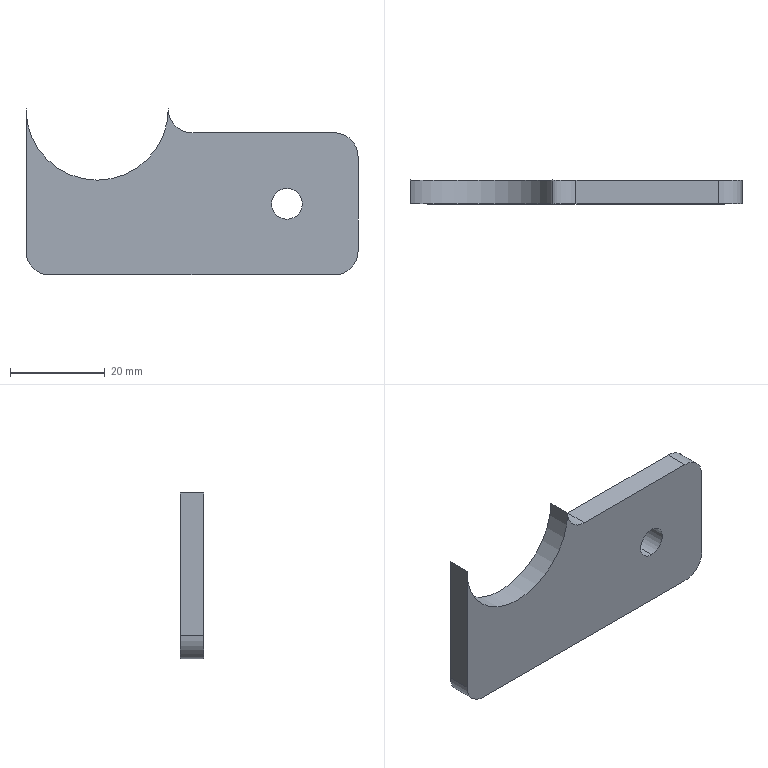Part | SolidWorks | features Cut 1, Extrusion 1, Fillet 1, ICE 1 | 1 solid | 13 faces | box 70 x 5 x 35 mm | volume 9263 mm3 | cylinder 7 | plane 6 | commonest cylinder face diameters 10 x4 6.5 x2 30 x1
STEP:
#1=CARTESIAN_POINT('',(40.,205.,-23.25));
#2=VERTEX_POINT('',#1);
#3=CARTESIAN_POINT('',(40.,205.,-16.75));
#4=VERTEX_POINT('',#3);
#5=CARTESIAN_POINT('',(40.,205.,-20.));
#6=DIRECTION('',(0.,1.,0.));
#7=DIRECTION('',(0.,0.,1.));
#8=AXIS2_PLACEMENT_3D('',#5,#6,#7);
#9=CIRCLE('',#8,3.25);
#10=EDGE_CURVE('',#2,#4,#9,.T.);
#11=ORIENTED_EDGE('',*,*,#10,.F.);
#12=CARTESIAN_POINT('',(40.,210.,-23.25));
#13=VERTEX_POINT('',#12);
#14=CARTESIAN_POINT('',(40.,205.,-23.25));
#15=DIRECTION('',(0.,1.,0.));
#16=VECTOR('',#15,1000.);
#17=LINE('',#14,#16);
#18=EDGE_CURVE('',#2,#13,#17,.T.);
#19=ORIENTED_EDGE('',*,*,#18,.T.);
#20=CARTESIAN_POINT('',(40.,210.,-16.75));
#21=VERTEX_POINT('',#20);
#22=CARTESIAN_POINT('',(40.,210.,-20.));
#23=DIRECTION('',(0.,1.,0.));
#24=DIRECTION('',(0.,0.,1.));
#25=AXIS2_PLACEMENT_3D('',#22,#23,#24);
#26=CIRCLE('',#25,3.25);
#27=EDGE_CURVE('',#13,#21,#26,.T.);
#28=ORIENTED_EDGE('',*,*,#27,.T.);
#29=CARTESIAN_POINT('',(40.,205.,-16.75));
#30=DIRECTION('',(0.,1.,0.));
#31=VECTOR('',#30,1000.);
#32=LINE('',#29,#31);
#33=EDGE_CURVE('',#4,#21,#32,.T.);
#34=ORIENTED_EDGE('',*,*,#33,.F.);
#35=EDGE_LOOP('',(#11,#19,#28,#34));
#36=FACE_OUTER_BOUND('',#35,.T.);
#37=CARTESIAN_POINT('',(40.,205.,-20.));
#38=DIRECTION('',(0.,1.,0.));
#39=DIRECTION('',(0.,0.,1.));
#40=AXIS2_PLACEMENT_3D('',#37,#38,#39);
#41=CYLINDRICAL_SURFACE('',#40,3.25);
#42=ADVANCED_FACE('',(#36),#41,.F.);
#43=CARTESIAN_POINT('',(20.,210.,-5.));
#44=VERTEX_POINT('',#43);
#45=CARTESIAN_POINT('',(50.,210.,-5.));
#46=VERTEX_POINT('',#45);
#47=CARTESIAN_POINT('',(14.142,210.,-5.));
#48=DIRECTION('',(1.,0.,0.));
#49=VECTOR('',#48,1000.);
#50=LINE('',#47,#49);
#51=EDGE_CURVE('',#44,#46,#50,.T.);
#52=ORIENTED_EDGE('',*,*,#51,.F.);
#53=CARTESIAN_POINT('',(20.,205.,-5.));
#54=VERTEX_POINT('',#53);
#55=CARTESIAN_POINT('',(20.,205.,-5.));
#56=DIRECTION('',(0.,1.,0.));
#57=VECTOR('',#56,1000.);
#58=LINE('',#55,#57);
#59=EDGE_CURVE('',#54,#44,#58,.T.);
#60=ORIENTED_EDGE('',*,*,#59,.F.);
#61=CARTESIAN_POINT('',(50.,205.,-5.));
#62=VERTEX_POINT('',#61);
#63=CARTESIAN_POINT('',(14.142,205.,-5.));
#64=DIRECTION('',(1.,0.,0.));
#65=VECTOR('',#64,1000.);
#66=LINE('',#63,#65);
#67=EDGE_CURVE('',#54,#62,#66,.T.);
#68=ORIENTED_EDGE('',*,*,#67,.T.);
#69=CARTESIAN_POINT('',(50.,205.,-5.));
#70=DIRECTION('',(0.,1.,0.));
#71=VECTOR('',#70,1000.);
#72=LINE('',#69,#71);
#73=EDGE_CURVE('',#62,#46,#72,.T.);
#74=ORIENTED_EDGE('',*,*,#73,.T.);
#75=EDGE_LOOP('',(#52,#60,#68,#74));
#76=FACE_OUTER_BOUND('',#75,.T.);
#77=CARTESIAN_POINT('',(14.142,205.,-5.));
#78=DIRECTION('',(0.,0.,1.));
#79=DIRECTION('',(1.,0.,0.));
#80=AXIS2_PLACEMENT_3D('',#77,#78,#79);
#81=PLANE('',#80);
#82=ADVANCED_FACE('',(#76),#81,.T.);
#83=CARTESIAN_POINT('',(-15.,210.,0.));
#84=VERTEX_POINT('',#83);
#85=CARTESIAN_POINT('',(15.,210.,0.));
#86=VERTEX_POINT('',#85);
#87=CARTESIAN_POINT('',(0.,210.,0.));
#88=DIRECTION('',(0.,-1.,0.));
#89=DIRECTION('',(0.,0.,1.));
#90=AXIS2_PLACEMENT_3D('',#87,#88,#89);
#91=CIRCLE('',#90,15.);
#92=EDGE_CURVE('',#84,#86,#91,.T.);
#93=ORIENTED_EDGE('',*,*,#92,.F.);
#94=CARTESIAN_POINT('',(-15.,205.,0.));
#95=VERTEX_POINT('',#94);
#96=CARTESIAN_POINT('',(-15.,205.,0.));
#97=DIRECTION('',(0.,1.,0.));
#98=VECTOR('',#97,1000.);
#99=LINE('',#96,#98);
#100=EDGE_CURVE('',#95,#84,#99,.T.);
#101=ORIENTED_EDGE('',*,*,#100,.F.);
#102=CARTESIAN_POINT('',(15.,205.,0.));
#103=VERTEX_POINT('',#102);
#104=CARTESIAN_POINT('',(0.,205.,0.));
#105=DIRECTION('',(0.,-1.,0.));
#106=DIRECTION('',(0.,0.,1.));
#107=AXIS2_PLACEMENT_3D('',#104,#105,#106);
#108=CIRCLE('',#107,15.);
#109=EDGE_CURVE('',#95,#103,#108,.T.);
#110=ORIENTED_EDGE('',*,*,#109,.T.);
#111=CARTESIAN_POINT('',(15.,205.,0.));
#112=DIRECTION('',(0.,1.,0.));
#113=VECTOR('',#112,1000.);
#114=LINE('',#111,#113);
#115=EDGE_CURVE('',#103,#86,#114,.T.);
#116=ORIENTED_EDGE('',*,*,#115,.T.);
#117=EDGE_LOOP('',(#93,#101,#110,#116));
#118=FACE_OUTER_BOUND('',#117,.T.);
#119=CARTESIAN_POINT('',(0.,205.,0.));
#120=DIRECTION('',(0.,1.,0.));
#121=DIRECTION('',(0.,0.,1.));
#122=AXIS2_PLACEMENT_3D('',#119,#120,#121);
#123=CYLINDRICAL_SURFACE('',#122,15.);
#124=ADVANCED_FACE('',(#118),#123,.F.);
#125=CARTESIAN_POINT('',(-15.,210.,-30.));
#126=VERTEX_POINT('',#125);
#127=CARTESIAN_POINT('',(-15.,210.,0.));
#128=DIRECTION('',(0.,0.,1.));
#129=VECTOR('',#128,1000.);
#130=LINE('',#127,#129);
#131=EDGE_CURVE('',#126,#84,#130,.T.);
#132=ORIENTED_EDGE('',*,*,#131,.F.);
#133=CARTESIAN_POINT('',(-15.,205.,-30.));
#134=VERTEX_POINT('',#133);
#135=CARTESIAN_POINT('',(-15.,205.,-30.));
#136=DIRECTION('',(0.,-1.,0.));
#137=VECTOR('',#136,1000.);
#138=LINE('',#135,#137);
#139=EDGE_CURVE('',#126,#134,#138,.T.);
#140=ORIENTED_EDGE('',*,*,#139,.T.);
#141=CARTESIAN_POINT('',(-15.,205.,0.));
#142=DIRECTION('',(0.,0.,1.));
#143=VECTOR('',#142,1000.);
#144=LINE('',#141,#143);
#145=EDGE_CURVE('',#134,#95,#144,.T.);
#146=ORIENTED_EDGE('',*,*,#145,.T.);
#147=ORIENTED_EDGE('',*,*,#100,.T.);
#148=EDGE_LOOP('',(#132,#140,#146,#147));
#149=FACE_OUTER_BOUND('',#148,.T.);
#150=CARTESIAN_POINT('',(-15.,205.,0.));
#151=DIRECTION('',(-1.,0.,0.));
#152=DIRECTION('',(0.,0.,1.));
#153=AXIS2_PLACEMENT_3D('',#150,#151,#152);
#154=PLANE('',#153);
#155=ADVANCED_FACE('',(#149),#154,.T.);
#156=CARTESIAN_POINT('',(50.,205.,-35.));
#157=VERTEX_POINT('',#156);
#158=CARTESIAN_POINT('',(-10.,205.,-35.));
#159=VERTEX_POINT('',#158);
#160=CARTESIAN_POINT('',(-15.,205.,-35.));
#161=DIRECTION('',(-1.,0.,0.));
#162=VECTOR('',#161,1000.);
#163=LINE('',#160,#162);
#164=EDGE_CURVE('',#157,#159,#163,.T.);
#165=ORIENTED_EDGE('',*,*,#164,.T.);
#166=CARTESIAN_POINT('',(-10.,210.,-35.));
#167=VERTEX_POINT('',#166);
#168=CARTESIAN_POINT('',(-10.,205.,-35.));
#169=DIRECTION('',(0.,1.,0.));
#170=VECTOR('',#169,1000.);
#171=LINE('',#168,#170);
#172=EDGE_CURVE('',#159,#167,#171,.T.);
#173=ORIENTED_EDGE('',*,*,#172,.T.);
#174=CARTESIAN_POINT('',(50.,210.,-35.));
#175=VERTEX_POINT('',#174);
#176=CARTESIAN_POINT('',(-15.,210.,-35.));
#177=DIRECTION('',(-1.,0.,0.));
#178=VECTOR('',#177,1000.);
#179=LINE('',#176,#178);
#180=EDGE_CURVE('',#175,#167,#179,.T.);
#181=ORIENTED_EDGE('',*,*,#180,.F.);
#182=CARTESIAN_POINT('',(50.,205.,-35.));
#183=DIRECTION('',(0.,-1.,0.));
#184=VECTOR('',#183,1000.);
#185=LINE('',#182,#184);
#186=EDGE_CURVE('',#175,#157,#185,.T.);
#187=ORIENTED_EDGE('',*,*,#186,.T.);
#188=EDGE_LOOP('',(#165,#173,#181,#187));
#189=FACE_OUTER_BOUND('',#188,.T.);
#190=CARTESIAN_POINT('',(-15.,205.,-35.));
#191=DIRECTION('',(0.,0.,-1.));
#192=DIRECTION('',(-1.,0.,0.));
#193=AXIS2_PLACEMENT_3D('',#190,#191,#192);
#194=PLANE('',#193);
#195=ADVANCED_FACE('',(#189),#194,.T.);
#196=CARTESIAN_POINT('',(55.,210.,-10.));
#197=VERTEX_POINT('',#196);
#198=CARTESIAN_POINT('',(55.,210.,-30.));
#199=VERTEX_POINT('',#198);
#200=CARTESIAN_POINT('',(55.,210.,-5.));
#201=DIRECTION('',(0.,0.,-1.));
#202=VECTOR('',#201,1000.);
#203=LINE('',#200,#202);
#204=EDGE_CURVE('',#197,#199,#203,.T.);
#205=ORIENTED_EDGE('',*,*,#204,.F.);
#206=CARTESIAN_POINT('',(55.,205.,-10.));
#207=VERTEX_POINT('',#206);
#208=CARTESIAN_POINT('',(55.,205.,-10.));
#209=DIRECTION('',(0.,-1.,0.));
#210=VECTOR('',#209,1000.);
#211=LINE('',#208,#210);
#212=EDGE_CURVE('',#197,#207,#211,.T.);
#213=ORIENTED_EDGE('',*,*,#212,.T.);
#214=CARTESIAN_POINT('',(55.,205.,-30.));
#215=VERTEX_POINT('',#214);
#216=CARTESIAN_POINT('',(55.,205.,-5.));
#217=DIRECTION('',(0.,0.,-1.));
#218=VECTOR('',#217,1000.);
#219=LINE('',#216,#218);
#220=EDGE_CURVE('',#207,#215,#219,.T.);
#221=ORIENTED_EDGE('',*,*,#220,.T.);
#222=CARTESIAN_POINT('',(55.,205.,-30.));
#223=DIRECTION('',(0.,1.,0.));
#224=VECTOR('',#223,1000.);
#225=LINE('',#222,#224);
#226=EDGE_CURVE('',#215,#199,#225,.T.);
#227=ORIENTED_EDGE('',*,*,#226,.T.);
#228=EDGE_LOOP('',(#205,#213,#221,#227));
#229=FACE_OUTER_BOUND('',#228,.T.);
#230=CARTESIAN_POINT('',(55.,205.,-5.));
#231=DIRECTION('',(1.,0.,0.));
#232=DIRECTION('',(0.,0.,-1.));
#233=AXIS2_PLACEMENT_3D('',#230,#231,#232);
#234=PLANE('',#233);
#235=ADVANCED_FACE('',(#229),#234,.T.);
#236=CARTESIAN_POINT('',(40.,205.,-20.));
#237=DIRECTION('',(0.,1.,0.));
#238=DIRECTION('',(0.,0.,1.));
#239=AXIS2_PLACEMENT_3D('',#236,#237,#238);
#240=CIRCLE('',#239,3.25);
#241=EDGE_CURVE('',#4,#2,#240,.T.);
#242=ORIENTED_EDGE('',*,*,#241,.T.);
#243=ORIENTED_EDGE('',*,*,#10,.T.);
#244=EDGE_LOOP('',(#242,#243));
#245=FACE_BOUND('',#244,.T.);
#246=ORIENTED_EDGE('',*,*,#220,.F.);
#247=CARTESIAN_POINT('',(50.,205.,-10.));
#248=DIRECTION('',(0.,-1.,0.));
#249=DIRECTION('',(0.,0.,1.));
#250=AXIS2_PLACEMENT_3D('',#247,#248,#249);
#251=CIRCLE('',#250,5.);
#252=EDGE_CURVE('',#207,#62,#251,.T.);
#253=ORIENTED_EDGE('',*,*,#252,.T.);
#254=ORIENTED_EDGE('',*,*,#67,.F.);
#255=CARTESIAN_POINT('',(20.,205.,0.));
#256=DIRECTION('',(0.,-1.,0.));
#257=DIRECTION('',(0.,0.,1.));
#258=AXIS2_PLACEMENT_3D('',#255,#256,#257);
#259=CIRCLE('',#258,5.);
#260=EDGE_CURVE('',#103,#54,#259,.T.);
#261=ORIENTED_EDGE('',*,*,#260,.F.);
#262=ORIENTED_EDGE('',*,*,#109,.F.);
#263=ORIENTED_EDGE('',*,*,#145,.F.);
#264=CARTESIAN_POINT('',(-10.,205.,-30.));
#265=DIRECTION('',(0.,-1.,0.));
#266=DIRECTION('',(0.,0.,1.));
#267=AXIS2_PLACEMENT_3D('',#264,#265,#266);
#268=CIRCLE('',#267,5.);
#269=EDGE_CURVE('',#134,#159,#268,.T.);
#270=ORIENTED_EDGE('',*,*,#269,.T.);
#271=ORIENTED_EDGE('',*,*,#164,.F.);
#272=CARTESIAN_POINT('',(50.,205.,-30.));
#273=DIRECTION('',(0.,-1.,0.));
#274=DIRECTION('',(0.,0.,1.));
#275=AXIS2_PLACEMENT_3D('',#272,#273,#274);
#276=CIRCLE('',#275,5.);
#277=EDGE_CURVE('',#157,#215,#276,.T.);
#278=ORIENTED_EDGE('',*,*,#277,.T.);
#279=EDGE_LOOP('',(#246,#253,#254,#261,#262,#263,#270,#271,#278));
#280=FACE_OUTER_BOUND('',#279,.T.);
#281=CARTESIAN_POINT('',(0.,205.,0.));
#282=DIRECTION('',(0.,1.,0.));
#283=DIRECTION('',(0.,0.,1.));
#284=AXIS2_PLACEMENT_3D('',#281,#282,#283);
#285=PLANE('',#284);
#286=ADVANCED_FACE('',(#245,#280),#285,.F.);
#287=CARTESIAN_POINT('',(40.,210.,-20.));
#288=DIRECTION('',(0.,1.,0.));
#289=DIRECTION('',(0.,0.,1.));
#290=AXIS2_PLACEMENT_3D('',#287,#288,#289);
#291=CIRCLE('',#290,3.25);
#292=EDGE_CURVE('',#21,#13,#291,.T.);
#293=ORIENTED_EDGE('',*,*,#292,.F.);
#294=ORIENTED_EDGE('',*,*,#27,.F.);
#295=EDGE_LOOP('',(#293,#294));
#296=FACE_BOUND('',#295,.T.);
#297=ORIENTED_EDGE('',*,*,#92,.T.);
#298=CARTESIAN_POINT('',(20.,210.,0.));
#299=DIRECTION('',(0.,-1.,0.));
#300=DIRECTION('',(0.,0.,1.));
#301=AXIS2_PLACEMENT_3D('',#298,#299,#300);
#302=CIRCLE('',#301,5.);
#303=EDGE_CURVE('',#86,#44,#302,.T.);
#304=ORIENTED_EDGE('',*,*,#303,.T.);
#305=ORIENTED_EDGE('',*,*,#51,.T.);
#306=CARTESIAN_POINT('',(50.,210.,-10.));
#307=DIRECTION('',(0.,1.,0.));
#308=DIRECTION('',(0.,0.,1.));
#309=AXIS2_PLACEMENT_3D('',#306,#307,#308);
#310=CIRCLE('',#309,5.);
#311=EDGE_CURVE('',#46,#197,#310,.T.);
#312=ORIENTED_EDGE('',*,*,#311,.T.);
#313=ORIENTED_EDGE('',*,*,#204,.T.);
#314=CARTESIAN_POINT('',(50.,210.,-30.));
#315=DIRECTION('',(0.,1.,0.));
#316=DIRECTION('',(0.,0.,1.));
#317=AXIS2_PLACEMENT_3D('',#314,#315,#316);
#318=CIRCLE('',#317,5.);
#319=EDGE_CURVE('',#199,#175,#318,.T.);
#320=ORIENTED_EDGE('',*,*,#319,.T.);
#321=ORIENTED_EDGE('',*,*,#180,.T.);
#322=CARTESIAN_POINT('',(-10.,210.,-30.));
#323=DIRECTION('',(0.,1.,0.));
#324=DIRECTION('',(0.,0.,1.));
#325=AXIS2_PLACEMENT_3D('',#322,#323,#324);
#326=CIRCLE('',#325,5.);
#327=EDGE_CURVE('',#167,#126,#326,.T.);
#328=ORIENTED_EDGE('',*,*,#327,.T.);
#329=ORIENTED_EDGE('',*,*,#131,.T.);
#330=EDGE_LOOP('',(#297,#304,#305,#312,#313,#320,#321,#328,#329));
#331=FACE_OUTER_BOUND('',#330,.T.);
#332=CARTESIAN_POINT('',(0.,210.,0.));
#333=DIRECTION('',(0.,1.,0.));
#334=DIRECTION('',(0.,0.,1.));
#335=AXIS2_PLACEMENT_3D('',#332,#333,#334);
#336=PLANE('',#335);
#337=ADVANCED_FACE('',(#296,#331),#336,.T.);
#338=ORIENTED_EDGE('',*,*,#252,.F.);
#339=ORIENTED_EDGE('',*,*,#212,.F.);
#340=ORIENTED_EDGE('',*,*,#311,.F.);
#341=ORIENTED_EDGE('',*,*,#73,.F.);
#342=EDGE_LOOP('',(#338,#339,#340,#341));
#343=FACE_OUTER_BOUND('',#342,.T.);
#344=CARTESIAN_POINT('',(50.,205.,-10.));
#345=DIRECTION('',(0.,1.,0.));
#346=DIRECTION('',(0.,0.,1.));
#347=AXIS2_PLACEMENT_3D('',#344,#345,#346);
#348=CYLINDRICAL_SURFACE('',#347,5.);
#349=ADVANCED_FACE('',(#343),#348,.T.);
#350=ORIENTED_EDGE('',*,*,#269,.F.);
#351=ORIENTED_EDGE('',*,*,#139,.F.);
#352=ORIENTED_EDGE('',*,*,#327,.F.);
#353=ORIENTED_EDGE('',*,*,#172,.F.);
#354=EDGE_LOOP('',(#350,#351,#352,#353));
#355=FACE_OUTER_BOUND('',#354,.T.);
#356=CARTESIAN_POINT('',(-10.,205.,-30.));
#357=DIRECTION('',(0.,1.,0.));
#358=DIRECTION('',(0.,0.,1.));
#359=AXIS2_PLACEMENT_3D('',#356,#357,#358);
#360=CYLINDRICAL_SURFACE('',#359,5.);
#361=ADVANCED_FACE('',(#355),#360,.T.);
#362=ORIENTED_EDGE('',*,*,#277,.F.);
#363=ORIENTED_EDGE('',*,*,#186,.F.);
#364=ORIENTED_EDGE('',*,*,#319,.F.);
#365=ORIENTED_EDGE('',*,*,#226,.F.);
#366=EDGE_LOOP('',(#362,#363,#364,#365));
#367=FACE_OUTER_BOUND('',#366,.T.);
#368=CARTESIAN_POINT('',(50.,205.,-30.));
#369=DIRECTION('',(0.,1.,0.));
#370=DIRECTION('',(0.,0.,1.));
#371=AXIS2_PLACEMENT_3D('',#368,#369,#370);
#372=CYLINDRICAL_SURFACE('',#371,5.);
#373=ADVANCED_FACE('',(#367),#372,.T.);
#374=ORIENTED_EDGE('',*,*,#18,.F.);
#375=ORIENTED_EDGE('',*,*,#241,.F.);
#376=ORIENTED_EDGE('',*,*,#33,.T.);
#377=ORIENTED_EDGE('',*,*,#292,.T.);
#378=EDGE_LOOP('',(#374,#375,#376,#377));
#379=FACE_OUTER_BOUND('',#378,.T.);
#380=CARTESIAN_POINT('',(40.,205.,-20.));
#381=DIRECTION('',(0.,1.,0.));
#382=DIRECTION('',(0.,0.,1.));
#383=AXIS2_PLACEMENT_3D('',#380,#381,#382);
#384=CYLINDRICAL_SURFACE('',#383,3.25);
#385=ADVANCED_FACE('',(#379),#384,.F.);
#386=ORIENTED_EDGE('',*,*,#303,.F.);
#387=ORIENTED_EDGE('',*,*,#115,.F.);
#388=ORIENTED_EDGE('',*,*,#260,.T.);
#389=ORIENTED_EDGE('',*,*,#59,.T.);
#390=EDGE_LOOP('',(#386,#387,#388,#389));
#391=FACE_OUTER_BOUND('',#390,.T.);
#392=CARTESIAN_POINT('',(20.,205.,0.));
#393=DIRECTION('',(0.,1.,0.));
#394=DIRECTION('',(0.,0.,1.));
#395=AXIS2_PLACEMENT_3D('',#392,#393,#394);
#396=CYLINDRICAL_SURFACE('',#395,5.);
#397=ADVANCED_FACE('',(#391),#396,.F.);
#398=CLOSED_SHELL('',(#42,#82,#124,#155,#195,#235,#286,#337,#349,#361,#373,#385,#397));
#399=MANIFOLD_SOLID_BREP('',#398);
#400=CARTESIAN_POINT('',(0.,0.,0.));
#401=DIRECTION('',(0.,0.,1.));
#402=DIRECTION('',(1.,0.,0.));
#403=AXIS2_PLACEMENT_3D('',#400,#401,#402);
#404=(LENGTH_UNIT()NAMED_UNIT(*)SI_UNIT(.MILLI.,.METRE.));
#405=UNCERTAINTY_MEASURE_WITH_UNIT(LENGTH_MEASURE(0.00001),#404,'','');
#406=(NAMED_UNIT(*)PLANE_ANGLE_UNIT()SI_UNIT($,.RADIAN.));
#407=(NAMED_UNIT(*)SI_UNIT($,.STERADIAN.)SOLID_ANGLE_UNIT());
#408=(GEOMETRIC_REPRESENTATION_CONTEXT(3)GLOBAL_UNCERTAINTY_ASSIGNED_CONTEXT((#405))GLOBAL_UNIT_ASSIGNED_CONTEXT((#404,#406,#407))REPRESENTATION_CONTEXT('',''));
#409=ADVANCED_BREP_SHAPE_REPRESENTATION('',(#399,#403),#408);